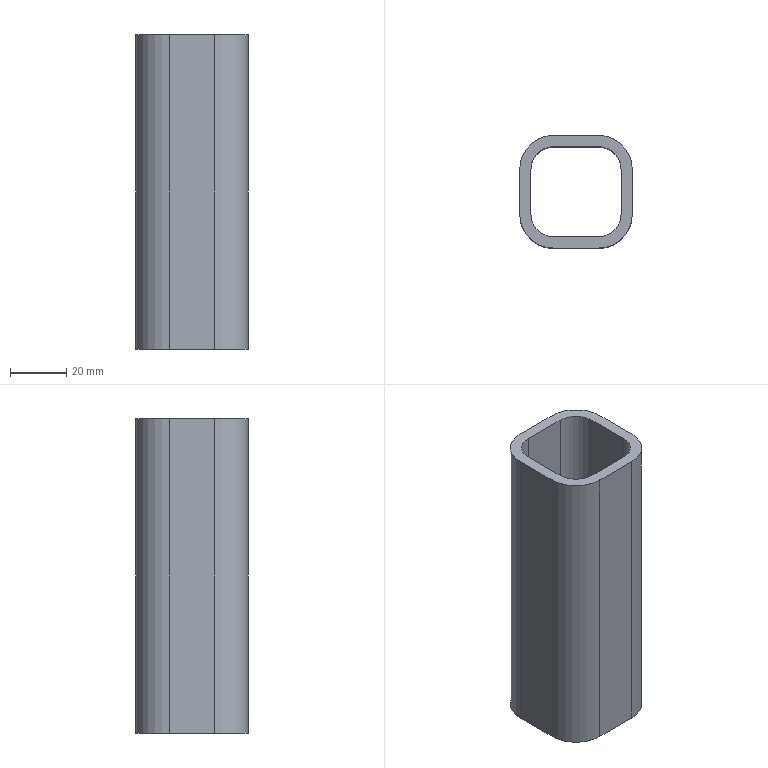Part | SolidWorks | features BaseBody 1 | 1 solid | 18 faces | box 40 x 40 x 111.5 mm | volume 56567 mm3 | plane 10 | cylinder 8 | commonest cylinder face diameters 16 x4 24 x4
STEP:
#1=CARTESIAN_POINT('',(8.,-20.,-31.5));
#2=VERTEX_POINT('',#1);
#3=CARTESIAN_POINT('',(20.,-8.,-31.5));
#4=VERTEX_POINT('',#3);
#5=CARTESIAN_POINT('',(8.,-8.,-31.5));
#6=DIRECTION('',(0.,0.,1.));
#7=DIRECTION('',(1.,0.,0.));
#8=AXIS2_PLACEMENT_3D('',#5,#6,#7);
#9=CIRCLE('',#8,12.);
#10=EDGE_CURVE('',#2,#4,#9,.T.);
#11=ORIENTED_EDGE('',*,*,#10,.T.);
#12=CARTESIAN_POINT('',(20.,-8.,80.));
#13=VERTEX_POINT('',#12);
#14=CARTESIAN_POINT('',(20.,-8.,0.));
#15=DIRECTION('',(0.,0.,1.));
#16=VECTOR('',#15,1000.);
#17=LINE('',#14,#16);
#18=EDGE_CURVE('',#4,#13,#17,.T.);
#19=ORIENTED_EDGE('',*,*,#18,.T.);
#20=CARTESIAN_POINT('',(8.,-20.,80.));
#21=VERTEX_POINT('',#20);
#22=CARTESIAN_POINT('',(8.,-8.,80.));
#23=DIRECTION('',(0.,0.,-1.));
#24=DIRECTION('',(1.,0.,0.));
#25=AXIS2_PLACEMENT_3D('',#22,#23,#24);
#26=CIRCLE('',#25,12.);
#27=EDGE_CURVE('',#13,#21,#26,.T.);
#28=ORIENTED_EDGE('',*,*,#27,.T.);
#29=CARTESIAN_POINT('',(8.,-20.,0.));
#30=DIRECTION('',(0.,0.,-1.));
#31=VECTOR('',#30,1000.);
#32=LINE('',#29,#31);
#33=EDGE_CURVE('',#21,#2,#32,.T.);
#34=ORIENTED_EDGE('',*,*,#33,.T.);
#35=EDGE_LOOP('',(#11,#19,#28,#34));
#36=FACE_OUTER_BOUND('',#35,.T.);
#37=CARTESIAN_POINT('',(8.,-8.,0.));
#38=DIRECTION('',(0.,0.,1.));
#39=DIRECTION('',(1.,0.,0.));
#40=AXIS2_PLACEMENT_3D('',#37,#38,#39);
#41=CYLINDRICAL_SURFACE('',#40,12.);
#42=ADVANCED_FACE('',(#36),#41,.T.);
#43=CARTESIAN_POINT('',(20.,8.,-31.5));
#44=VERTEX_POINT('',#43);
#45=CARTESIAN_POINT('',(20.,8.,-31.5));
#46=DIRECTION('',(0.,1.,0.));
#47=VECTOR('',#46,1000.);
#48=LINE('',#45,#47);
#49=EDGE_CURVE('',#4,#44,#48,.T.);
#50=ORIENTED_EDGE('',*,*,#49,.T.);
#51=CARTESIAN_POINT('',(20.,8.,80.));
#52=VERTEX_POINT('',#51);
#53=CARTESIAN_POINT('',(20.,8.,0.));
#54=DIRECTION('',(0.,0.,1.));
#55=VECTOR('',#54,1000.);
#56=LINE('',#53,#55);
#57=EDGE_CURVE('',#44,#52,#56,.T.);
#58=ORIENTED_EDGE('',*,*,#57,.T.);
#59=CARTESIAN_POINT('',(20.,8.,80.));
#60=DIRECTION('',(0.,-1.,0.));
#61=VECTOR('',#60,1000.);
#62=LINE('',#59,#61);
#63=EDGE_CURVE('',#52,#13,#62,.T.);
#64=ORIENTED_EDGE('',*,*,#63,.T.);
#65=ORIENTED_EDGE('',*,*,#18,.F.);
#66=EDGE_LOOP('',(#50,#58,#64,#65));
#67=FACE_OUTER_BOUND('',#66,.T.);
#68=CARTESIAN_POINT('',(20.,8.,0.));
#69=DIRECTION('',(1.,0.,0.));
#70=DIRECTION('',(0.,1.,0.));
#71=AXIS2_PLACEMENT_3D('',#68,#69,#70);
#72=PLANE('',#71);
#73=ADVANCED_FACE('',(#67),#72,.T.);
#74=CARTESIAN_POINT('',(-16.,8.,-31.5));
#75=VERTEX_POINT('',#74);
#76=CARTESIAN_POINT('',(-8.,16.,-31.5));
#77=VERTEX_POINT('',#76);
#78=CARTESIAN_POINT('',(-8.,8.,-31.5));
#79=DIRECTION('',(0.,0.,-1.));
#80=DIRECTION('',(1.,0.,0.));
#81=AXIS2_PLACEMENT_3D('',#78,#79,#80);
#82=CIRCLE('',#81,8.);
#83=EDGE_CURVE('',#75,#77,#82,.T.);
#84=ORIENTED_EDGE('',*,*,#83,.F.);
#85=CARTESIAN_POINT('',(-16.,-8.,-31.5));
#86=VERTEX_POINT('',#85);
#87=CARTESIAN_POINT('',(-16.,0.,-31.5));
#88=DIRECTION('',(0.,1.,0.));
#89=VECTOR('',#88,1000.);
#90=LINE('',#87,#89);
#91=EDGE_CURVE('',#86,#75,#90,.T.);
#92=ORIENTED_EDGE('',*,*,#91,.F.);
#93=CARTESIAN_POINT('',(-8.,-16.,-31.5));
#94=VERTEX_POINT('',#93);
#95=CARTESIAN_POINT('',(-8.,-8.,-31.5));
#96=DIRECTION('',(0.,0.,-1.));
#97=DIRECTION('',(1.,0.,0.));
#98=AXIS2_PLACEMENT_3D('',#95,#96,#97);
#99=CIRCLE('',#98,8.);
#100=EDGE_CURVE('',#94,#86,#99,.T.);
#101=ORIENTED_EDGE('',*,*,#100,.F.);
#102=CARTESIAN_POINT('',(8.,-16.,-31.5));
#103=VERTEX_POINT('',#102);
#104=CARTESIAN_POINT('',(0.,-16.,-31.5));
#105=DIRECTION('',(-1.,0.,0.));
#106=VECTOR('',#105,1000.);
#107=LINE('',#104,#106);
#108=EDGE_CURVE('',#103,#94,#107,.T.);
#109=ORIENTED_EDGE('',*,*,#108,.F.);
#110=CARTESIAN_POINT('',(16.,-8.,-31.5));
#111=VERTEX_POINT('',#110);
#112=CARTESIAN_POINT('',(8.,-8.,-31.5));
#113=DIRECTION('',(0.,0.,-1.));
#114=DIRECTION('',(1.,0.,0.));
#115=AXIS2_PLACEMENT_3D('',#112,#113,#114);
#116=CIRCLE('',#115,8.);
#117=EDGE_CURVE('',#111,#103,#116,.T.);
#118=ORIENTED_EDGE('',*,*,#117,.F.);
#119=CARTESIAN_POINT('',(16.,8.,-31.5));
#120=VERTEX_POINT('',#119);
#121=CARTESIAN_POINT('',(16.,0.,-31.5));
#122=DIRECTION('',(0.,-1.,0.));
#123=VECTOR('',#122,1000.);
#124=LINE('',#121,#123);
#125=EDGE_CURVE('',#120,#111,#124,.T.);
#126=ORIENTED_EDGE('',*,*,#125,.F.);
#127=CARTESIAN_POINT('',(8.,16.,-31.5));
#128=VERTEX_POINT('',#127);
#129=CARTESIAN_POINT('',(8.,8.,-31.5));
#130=DIRECTION('',(0.,0.,-1.));
#131=DIRECTION('',(1.,0.,0.));
#132=AXIS2_PLACEMENT_3D('',#129,#130,#131);
#133=CIRCLE('',#132,8.);
#134=EDGE_CURVE('',#128,#120,#133,.T.);
#135=ORIENTED_EDGE('',*,*,#134,.F.);
#136=CARTESIAN_POINT('',(0.,16.,-31.5));
#137=DIRECTION('',(1.,0.,0.));
#138=VECTOR('',#137,1000.);
#139=LINE('',#136,#138);
#140=EDGE_CURVE('',#77,#128,#139,.T.);
#141=ORIENTED_EDGE('',*,*,#140,.F.);
#142=EDGE_LOOP('',(#84,#92,#101,#109,#118,#126,#135,#141));
#143=FACE_BOUND('',#142,.T.);
#144=CARTESIAN_POINT('',(-8.,20.,-31.5));
#145=VERTEX_POINT('',#144);
#146=CARTESIAN_POINT('',(-20.,8.,-31.5));
#147=VERTEX_POINT('',#146);
#148=CARTESIAN_POINT('',(-8.,8.,-31.5));
#149=DIRECTION('',(0.,0.,1.));
#150=DIRECTION('',(1.,0.,0.));
#151=AXIS2_PLACEMENT_3D('',#148,#149,#150);
#152=CIRCLE('',#151,12.);
#153=EDGE_CURVE('',#145,#147,#152,.T.);
#154=ORIENTED_EDGE('',*,*,#153,.F.);
#155=CARTESIAN_POINT('',(8.,20.,-31.5));
#156=VERTEX_POINT('',#155);
#157=CARTESIAN_POINT('',(0.,20.,-31.5));
#158=DIRECTION('',(-1.,0.,0.));
#159=VECTOR('',#158,1000.);
#160=LINE('',#157,#159);
#161=EDGE_CURVE('',#156,#145,#160,.T.);
#162=ORIENTED_EDGE('',*,*,#161,.F.);
#163=CARTESIAN_POINT('',(8.,8.,-31.5));
#164=DIRECTION('',(0.,0.,1.));
#165=DIRECTION('',(1.,0.,0.));
#166=AXIS2_PLACEMENT_3D('',#163,#164,#165);
#167=CIRCLE('',#166,12.);
#168=EDGE_CURVE('',#44,#156,#167,.T.);
#169=ORIENTED_EDGE('',*,*,#168,.F.);
#170=ORIENTED_EDGE('',*,*,#49,.F.);
#171=ORIENTED_EDGE('',*,*,#10,.F.);
#172=CARTESIAN_POINT('',(-8.,-20.,-31.5));
#173=VERTEX_POINT('',#172);
#174=CARTESIAN_POINT('',(0.,-20.,-31.5));
#175=DIRECTION('',(1.,0.,0.));
#176=VECTOR('',#175,1000.);
#177=LINE('',#174,#176);
#178=EDGE_CURVE('',#173,#2,#177,.T.);
#179=ORIENTED_EDGE('',*,*,#178,.F.);
#180=CARTESIAN_POINT('',(-20.,-8.,-31.5));
#181=VERTEX_POINT('',#180);
#182=CARTESIAN_POINT('',(-8.,-8.,-31.5));
#183=DIRECTION('',(0.,0.,1.));
#184=DIRECTION('',(1.,0.,0.));
#185=AXIS2_PLACEMENT_3D('',#182,#183,#184);
#186=CIRCLE('',#185,12.);
#187=EDGE_CURVE('',#181,#173,#186,.T.);
#188=ORIENTED_EDGE('',*,*,#187,.F.);
#189=CARTESIAN_POINT('',(-20.,0.,-31.5));
#190=DIRECTION('',(0.,-1.,0.));
#191=VECTOR('',#190,1000.);
#192=LINE('',#189,#191);
#193=EDGE_CURVE('',#147,#181,#192,.T.);
#194=ORIENTED_EDGE('',*,*,#193,.F.);
#195=EDGE_LOOP('',(#154,#162,#169,#170,#171,#179,#188,#194));
#196=FACE_OUTER_BOUND('',#195,.T.);
#197=CARTESIAN_POINT('',(0.,0.,-31.5));
#198=DIRECTION('',(0.,0.,1.));
#199=DIRECTION('',(1.,0.,0.));
#200=AXIS2_PLACEMENT_3D('',#197,#198,#199);
#201=PLANE('',#200);
#202=ADVANCED_FACE('',(#143,#196),#201,.F.);
#203=ORIENTED_EDGE('',*,*,#178,.T.);
#204=ORIENTED_EDGE('',*,*,#33,.F.);
#205=CARTESIAN_POINT('',(-8.,-20.,80.));
#206=VERTEX_POINT('',#205);
#207=CARTESIAN_POINT('',(8.,-20.,80.));
#208=DIRECTION('',(-1.,0.,0.));
#209=VECTOR('',#208,1000.);
#210=LINE('',#207,#209);
#211=EDGE_CURVE('',#21,#206,#210,.T.);
#212=ORIENTED_EDGE('',*,*,#211,.T.);
#213=CARTESIAN_POINT('',(-8.,-20.,0.));
#214=DIRECTION('',(0.,0.,-1.));
#215=VECTOR('',#214,1000.);
#216=LINE('',#213,#215);
#217=EDGE_CURVE('',#206,#173,#216,.T.);
#218=ORIENTED_EDGE('',*,*,#217,.T.);
#219=EDGE_LOOP('',(#203,#204,#212,#218));
#220=FACE_OUTER_BOUND('',#219,.T.);
#221=CARTESIAN_POINT('',(8.,-20.,0.));
#222=DIRECTION('',(0.,-1.,0.));
#223=DIRECTION('',(1.,0.,0.));
#224=AXIS2_PLACEMENT_3D('',#221,#222,#223);
#225=PLANE('',#224);
#226=ADVANCED_FACE('',(#220),#225,.T.);
#227=CARTESIAN_POINT('',(-16.,-8.,80.));
#228=VERTEX_POINT('',#227);
#229=CARTESIAN_POINT('',(-16.,8.,80.));
#230=VERTEX_POINT('',#229);
#231=CARTESIAN_POINT('',(-16.,0.,80.));
#232=DIRECTION('',(0.,1.,0.));
#233=VECTOR('',#232,1000.);
#234=LINE('',#231,#233);
#235=EDGE_CURVE('',#228,#230,#234,.T.);
#236=ORIENTED_EDGE('',*,*,#235,.T.);
#237=CARTESIAN_POINT('',(-8.,16.,80.));
#238=VERTEX_POINT('',#237);
#239=CARTESIAN_POINT('',(-8.,8.,80.));
#240=DIRECTION('',(0.,0.,-1.));
#241=DIRECTION('',(1.,0.,0.));
#242=AXIS2_PLACEMENT_3D('',#239,#240,#241);
#243=CIRCLE('',#242,8.);
#244=EDGE_CURVE('',#230,#238,#243,.T.);
#245=ORIENTED_EDGE('',*,*,#244,.T.);
#246=CARTESIAN_POINT('',(8.,16.,80.));
#247=VERTEX_POINT('',#246);
#248=CARTESIAN_POINT('',(0.,16.,80.));
#249=DIRECTION('',(1.,0.,0.));
#250=VECTOR('',#249,1000.);
#251=LINE('',#248,#250);
#252=EDGE_CURVE('',#238,#247,#251,.T.);
#253=ORIENTED_EDGE('',*,*,#252,.T.);
#254=CARTESIAN_POINT('',(16.,8.,80.));
#255=VERTEX_POINT('',#254);
#256=CARTESIAN_POINT('',(8.,8.,80.));
#257=DIRECTION('',(0.,0.,-1.));
#258=DIRECTION('',(1.,0.,0.));
#259=AXIS2_PLACEMENT_3D('',#256,#257,#258);
#260=CIRCLE('',#259,8.);
#261=EDGE_CURVE('',#247,#255,#260,.T.);
#262=ORIENTED_EDGE('',*,*,#261,.T.);
#263=CARTESIAN_POINT('',(16.,-8.,80.));
#264=VERTEX_POINT('',#263);
#265=CARTESIAN_POINT('',(16.,0.,80.));
#266=DIRECTION('',(0.,-1.,0.));
#267=VECTOR('',#266,1000.);
#268=LINE('',#265,#267);
#269=EDGE_CURVE('',#255,#264,#268,.T.);
#270=ORIENTED_EDGE('',*,*,#269,.T.);
#271=CARTESIAN_POINT('',(8.,-16.,80.));
#272=VERTEX_POINT('',#271);
#273=CARTESIAN_POINT('',(8.,-8.,80.));
#274=DIRECTION('',(0.,0.,-1.));
#275=DIRECTION('',(1.,0.,0.));
#276=AXIS2_PLACEMENT_3D('',#273,#274,#275);
#277=CIRCLE('',#276,8.);
#278=EDGE_CURVE('',#264,#272,#277,.T.);
#279=ORIENTED_EDGE('',*,*,#278,.T.);
#280=CARTESIAN_POINT('',(-8.,-16.,80.));
#281=VERTEX_POINT('',#280);
#282=CARTESIAN_POINT('',(0.,-16.,80.));
#283=DIRECTION('',(-1.,0.,0.));
#284=VECTOR('',#283,1000.);
#285=LINE('',#282,#284);
#286=EDGE_CURVE('',#272,#281,#285,.T.);
#287=ORIENTED_EDGE('',*,*,#286,.T.);
#288=CARTESIAN_POINT('',(-8.,-8.,80.));
#289=DIRECTION('',(0.,0.,-1.));
#290=DIRECTION('',(1.,0.,0.));
#291=AXIS2_PLACEMENT_3D('',#288,#289,#290);
#292=CIRCLE('',#291,8.);
#293=EDGE_CURVE('',#281,#228,#292,.T.);
#294=ORIENTED_EDGE('',*,*,#293,.T.);
#295=EDGE_LOOP('',(#236,#245,#253,#262,#270,#279,#287,#294));
#296=FACE_BOUND('',#295,.T.);
#297=CARTESIAN_POINT('',(8.,20.,80.));
#298=VERTEX_POINT('',#297);
#299=CARTESIAN_POINT('',(-8.,20.,80.));
#300=VERTEX_POINT('',#299);
#301=CARTESIAN_POINT('',(0.,20.,80.));
#302=DIRECTION('',(-1.,0.,0.));
#303=VECTOR('',#302,1000.);
#304=LINE('',#301,#303);
#305=EDGE_CURVE('',#298,#300,#304,.T.);
#306=ORIENTED_EDGE('',*,*,#305,.T.);
#307=CARTESIAN_POINT('',(-20.,8.,80.));
#308=VERTEX_POINT('',#307);
#309=CARTESIAN_POINT('',(-8.,8.,80.));
#310=DIRECTION('',(0.,0.,1.));
#311=DIRECTION('',(1.,0.,0.));
#312=AXIS2_PLACEMENT_3D('',#309,#310,#311);
#313=CIRCLE('',#312,12.);
#314=EDGE_CURVE('',#300,#308,#313,.T.);
#315=ORIENTED_EDGE('',*,*,#314,.T.);
#316=CARTESIAN_POINT('',(-20.,-8.,80.));
#317=VERTEX_POINT('',#316);
#318=CARTESIAN_POINT('',(-20.,0.,80.));
#319=DIRECTION('',(0.,-1.,0.));
#320=VECTOR('',#319,1000.);
#321=LINE('',#318,#320);
#322=EDGE_CURVE('',#308,#317,#321,.T.);
#323=ORIENTED_EDGE('',*,*,#322,.T.);
#324=CARTESIAN_POINT('',(-8.,-8.,80.));
#325=DIRECTION('',(0.,0.,1.));
#326=DIRECTION('',(1.,0.,0.));
#327=AXIS2_PLACEMENT_3D('',#324,#325,#326);
#328=CIRCLE('',#327,12.);
#329=EDGE_CURVE('',#317,#206,#328,.T.);
#330=ORIENTED_EDGE('',*,*,#329,.T.);
#331=ORIENTED_EDGE('',*,*,#211,.F.);
#332=ORIENTED_EDGE('',*,*,#27,.F.);
#333=ORIENTED_EDGE('',*,*,#63,.F.);
#334=CARTESIAN_POINT('',(8.,8.,80.));
#335=DIRECTION('',(0.,0.,1.));
#336=DIRECTION('',(1.,0.,0.));
#337=AXIS2_PLACEMENT_3D('',#334,#335,#336);
#338=CIRCLE('',#337,12.);
#339=EDGE_CURVE('',#52,#298,#338,.T.);
#340=ORIENTED_EDGE('',*,*,#339,.T.);
#341=EDGE_LOOP('',(#306,#315,#323,#330,#331,#332,#333,#340));
#342=FACE_OUTER_BOUND('',#341,.T.);
#343=CARTESIAN_POINT('',(0.,0.,80.));
#344=DIRECTION('',(0.,0.,1.));
#345=DIRECTION('',(1.,0.,0.));
#346=AXIS2_PLACEMENT_3D('',#343,#344,#345);
#347=PLANE('',#346);
#348=ADVANCED_FACE('',(#296,#342),#347,.T.);
#349=ORIENTED_EDGE('',*,*,#168,.T.);
#350=CARTESIAN_POINT('',(8.,20.,0.));
#351=DIRECTION('',(0.,0.,1.));
#352=VECTOR('',#351,1000.);
#353=LINE('',#350,#352);
#354=EDGE_CURVE('',#156,#298,#353,.T.);
#355=ORIENTED_EDGE('',*,*,#354,.T.);
#356=ORIENTED_EDGE('',*,*,#339,.F.);
#357=ORIENTED_EDGE('',*,*,#57,.F.);
#358=EDGE_LOOP('',(#349,#355,#356,#357));
#359=FACE_OUTER_BOUND('',#358,.T.);
#360=CARTESIAN_POINT('',(8.,8.,0.));
#361=DIRECTION('',(0.,0.,1.));
#362=DIRECTION('',(1.,0.,0.));
#363=AXIS2_PLACEMENT_3D('',#360,#361,#362);
#364=CYLINDRICAL_SURFACE('',#363,12.);
#365=ADVANCED_FACE('',(#359),#364,.T.);
#366=CARTESIAN_POINT('',(-8.,16.,0.));
#367=DIRECTION('',(0.,0.,1.));
#368=VECTOR('',#367,1000.);
#369=LINE('',#366,#368);
#370=EDGE_CURVE('',#77,#238,#369,.T.);
#371=ORIENTED_EDGE('',*,*,#370,.F.);
#372=ORIENTED_EDGE('',*,*,#140,.T.);
#373=CARTESIAN_POINT('',(8.,16.,0.));
#374=DIRECTION('',(0.,0.,-1.));
#375=VECTOR('',#374,1000.);
#376=LINE('',#373,#375);
#377=EDGE_CURVE('',#247,#128,#376,.T.);
#378=ORIENTED_EDGE('',*,*,#377,.F.);
#379=ORIENTED_EDGE('',*,*,#252,.F.);
#380=EDGE_LOOP('',(#371,#372,#378,#379));
#381=FACE_OUTER_BOUND('',#380,.T.);
#382=CARTESIAN_POINT('',(-8.,16.,0.));
#383=DIRECTION('',(0.,1.,0.));
#384=DIRECTION('',(-1.,0.,0.));
#385=AXIS2_PLACEMENT_3D('',#382,#383,#384);
#386=PLANE('',#385);
#387=ADVANCED_FACE('',(#381),#386,.F.);
#388=CARTESIAN_POINT('',(-16.,8.,0.));
#389=DIRECTION('',(0.,0.,1.));
#390=VECTOR('',#389,1000.);
#391=LINE('',#388,#390);
#392=EDGE_CURVE('',#75,#230,#391,.T.);
#393=ORIENTED_EDGE('',*,*,#392,.F.);
#394=ORIENTED_EDGE('',*,*,#83,.T.);
#395=ORIENTED_EDGE('',*,*,#370,.T.);
#396=ORIENTED_EDGE('',*,*,#244,.F.);
#397=EDGE_LOOP('',(#393,#394,#395,#396));
#398=FACE_OUTER_BOUND('',#397,.T.);
#399=CARTESIAN_POINT('',(-8.,8.,0.));
#400=DIRECTION('',(0.,0.,1.));
#401=DIRECTION('',(1.,0.,0.));
#402=AXIS2_PLACEMENT_3D('',#399,#400,#401);
#403=CYLINDRICAL_SURFACE('',#402,8.);
#404=ADVANCED_FACE('',(#398),#403,.F.);
#405=CARTESIAN_POINT('',(-16.,-8.,0.));
#406=DIRECTION('',(0.,0.,1.));
#407=VECTOR('',#406,1000.);
#408=LINE('',#405,#407);
#409=EDGE_CURVE('',#86,#228,#408,.T.);
#410=ORIENTED_EDGE('',*,*,#409,.F.);
#411=ORIENTED_EDGE('',*,*,#91,.T.);
#412=ORIENTED_EDGE('',*,*,#392,.T.);
#413=ORIENTED_EDGE('',*,*,#235,.F.);
#414=EDGE_LOOP('',(#410,#411,#412,#413));
#415=FACE_OUTER_BOUND('',#414,.T.);
#416=CARTESIAN_POINT('',(-16.,-8.,0.));
#417=DIRECTION('',(-1.,0.,0.));
#418=DIRECTION('',(0.,-1.,0.));
#419=AXIS2_PLACEMENT_3D('',#416,#417,#418);
#420=PLANE('',#419);
#421=ADVANCED_FACE('',(#415),#420,.F.);
#422=CARTESIAN_POINT('',(-8.,-16.,0.));
#423=DIRECTION('',(0.,0.,1.));
#424=VECTOR('',#423,1000.);
#425=LINE('',#422,#424);
#426=EDGE_CURVE('',#94,#281,#425,.T.);
#427=ORIENTED_EDGE('',*,*,#426,.F.);
#428=ORIENTED_EDGE('',*,*,#100,.T.);
#429=ORIENTED_EDGE('',*,*,#409,.T.);
#430=ORIENTED_EDGE('',*,*,#293,.F.);
#431=EDGE_LOOP('',(#427,#428,#429,#430));
#432=FACE_OUTER_BOUND('',#431,.T.);
#433=CARTESIAN_POINT('',(-8.,-8.,0.));
#434=DIRECTION('',(0.,0.,1.));
#435=DIRECTION('',(1.,0.,0.));
#436=AXIS2_PLACEMENT_3D('',#433,#434,#435);
#437=CYLINDRICAL_SURFACE('',#436,8.);
#438=ADVANCED_FACE('',(#432),#437,.F.);
#439=CARTESIAN_POINT('',(8.,-16.,0.));
#440=DIRECTION('',(0.,0.,1.));
#441=VECTOR('',#440,1000.);
#442=LINE('',#439,#441);
#443=EDGE_CURVE('',#103,#272,#442,.T.);
#444=ORIENTED_EDGE('',*,*,#443,.F.);
#445=ORIENTED_EDGE('',*,*,#108,.T.);
#446=ORIENTED_EDGE('',*,*,#426,.T.);
#447=ORIENTED_EDGE('',*,*,#286,.F.);
#448=EDGE_LOOP('',(#444,#445,#446,#447));
#449=FACE_OUTER_BOUND('',#448,.T.);
#450=CARTESIAN_POINT('',(8.,-16.,0.));
#451=DIRECTION('',(0.,-1.,0.));
#452=DIRECTION('',(1.,0.,0.));
#453=AXIS2_PLACEMENT_3D('',#450,#451,#452);
#454=PLANE('',#453);
#455=ADVANCED_FACE('',(#449),#454,.F.);
#456=CARTESIAN_POINT('',(16.,-8.,0.));
#457=DIRECTION('',(0.,0.,1.));
#458=VECTOR('',#457,1000.);
#459=LINE('',#456,#458);
#460=EDGE_CURVE('',#111,#264,#459,.T.);
#461=ORIENTED_EDGE('',*,*,#460,.F.);
#462=ORIENTED_EDGE('',*,*,#117,.T.);
#463=ORIENTED_EDGE('',*,*,#443,.T.);
#464=ORIENTED_EDGE('',*,*,#278,.F.);
#465=EDGE_LOOP('',(#461,#462,#463,#464));
#466=FACE_OUTER_BOUND('',#465,.T.);
#467=CARTESIAN_POINT('',(8.,-8.,0.));
#468=DIRECTION('',(0.,0.,1.));
#469=DIRECTION('',(1.,0.,0.));
#470=AXIS2_PLACEMENT_3D('',#467,#468,#469);
#471=CYLINDRICAL_SURFACE('',#470,8.);
#472=ADVANCED_FACE('',(#466),#471,.F.);
#473=CARTESIAN_POINT('',(16.,8.,0.));
#474=DIRECTION('',(0.,0.,1.));
#475=VECTOR('',#474,1000.);
#476=LINE('',#473,#475);
#477=EDGE_CURVE('',#120,#255,#476,.T.);
#478=ORIENTED_EDGE('',*,*,#477,.F.);
#479=ORIENTED_EDGE('',*,*,#125,.T.);
#480=ORIENTED_EDGE('',*,*,#460,.T.);
#481=ORIENTED_EDGE('',*,*,#269,.F.);
#482=EDGE_LOOP('',(#478,#479,#480,#481));
#483=FACE_OUTER_BOUND('',#482,.T.);
#484=CARTESIAN_POINT('',(16.,8.,0.));
#485=DIRECTION('',(1.,0.,0.));
#486=DIRECTION('',(0.,0.,-1.));
#487=AXIS2_PLACEMENT_3D('',#484,#485,#486);
#488=PLANE('',#487);
#489=ADVANCED_FACE('',(#483),#488,.F.);
#490=ORIENTED_EDGE('',*,*,#377,.T.);
#491=ORIENTED_EDGE('',*,*,#134,.T.);
#492=ORIENTED_EDGE('',*,*,#477,.T.);
#493=ORIENTED_EDGE('',*,*,#261,.F.);
#494=EDGE_LOOP('',(#490,#491,#492,#493));
#495=FACE_OUTER_BOUND('',#494,.T.);
#496=CARTESIAN_POINT('',(8.,8.,0.));
#497=DIRECTION('',(0.,0.,1.));
#498=DIRECTION('',(1.,0.,0.));
#499=AXIS2_PLACEMENT_3D('',#496,#497,#498);
#500=CYLINDRICAL_SURFACE('',#499,8.);
#501=ADVANCED_FACE('',(#495),#500,.F.);
#502=ORIENTED_EDGE('',*,*,#193,.T.);
#503=CARTESIAN_POINT('',(-20.,-8.,0.));
#504=DIRECTION('',(0.,0.,1.));
#505=VECTOR('',#504,1000.);
#506=LINE('',#503,#505);
#507=EDGE_CURVE('',#181,#317,#506,.T.);
#508=ORIENTED_EDGE('',*,*,#507,.T.);
#509=ORIENTED_EDGE('',*,*,#322,.F.);
#510=CARTESIAN_POINT('',(-20.,8.,0.));
#511=DIRECTION('',(0.,0.,-1.));
#512=VECTOR('',#511,1000.);
#513=LINE('',#510,#512);
#514=EDGE_CURVE('',#308,#147,#513,.T.);
#515=ORIENTED_EDGE('',*,*,#514,.T.);
#516=EDGE_LOOP('',(#502,#508,#509,#515));
#517=FACE_OUTER_BOUND('',#516,.T.);
#518=CARTESIAN_POINT('',(-20.,-8.,0.));
#519=DIRECTION('',(-1.,0.,0.));
#520=DIRECTION('',(0.,-1.,0.));
#521=AXIS2_PLACEMENT_3D('',#518,#519,#520);
#522=PLANE('',#521);
#523=ADVANCED_FACE('',(#517),#522,.T.);
#524=ORIENTED_EDGE('',*,*,#153,.T.);
#525=ORIENTED_EDGE('',*,*,#514,.F.);
#526=ORIENTED_EDGE('',*,*,#314,.F.);
#527=CARTESIAN_POINT('',(-8.,20.,0.));
#528=DIRECTION('',(0.,0.,-1.));
#529=VECTOR('',#528,1000.);
#530=LINE('',#527,#529);
#531=EDGE_CURVE('',#300,#145,#530,.T.);
#532=ORIENTED_EDGE('',*,*,#531,.T.);
#533=EDGE_LOOP('',(#524,#525,#526,#532));
#534=FACE_OUTER_BOUND('',#533,.T.);
#535=CARTESIAN_POINT('',(-8.,8.,0.));
#536=DIRECTION('',(0.,0.,1.));
#537=DIRECTION('',(1.,0.,0.));
#538=AXIS2_PLACEMENT_3D('',#535,#536,#537);
#539=CYLINDRICAL_SURFACE('',#538,12.);
#540=ADVANCED_FACE('',(#534),#539,.T.);
#541=ORIENTED_EDGE('',*,*,#161,.T.);
#542=ORIENTED_EDGE('',*,*,#531,.F.);
#543=ORIENTED_EDGE('',*,*,#305,.F.);
#544=ORIENTED_EDGE('',*,*,#354,.F.);
#545=EDGE_LOOP('',(#541,#542,#543,#544));
#546=FACE_OUTER_BOUND('',#545,.T.);
#547=CARTESIAN_POINT('',(-8.,20.,0.));
#548=DIRECTION('',(0.,1.,0.));
#549=DIRECTION('',(0.,0.,1.));
#550=AXIS2_PLACEMENT_3D('',#547,#548,#549);
#551=PLANE('',#550);
#552=ADVANCED_FACE('',(#546),#551,.T.);
#553=ORIENTED_EDGE('',*,*,#187,.T.);
#554=ORIENTED_EDGE('',*,*,#217,.F.);
#555=ORIENTED_EDGE('',*,*,#329,.F.);
#556=ORIENTED_EDGE('',*,*,#507,.F.);
#557=EDGE_LOOP('',(#553,#554,#555,#556));
#558=FACE_OUTER_BOUND('',#557,.T.);
#559=CARTESIAN_POINT('',(-8.,-8.,0.));
#560=DIRECTION('',(0.,0.,1.));
#561=DIRECTION('',(1.,0.,0.));
#562=AXIS2_PLACEMENT_3D('',#559,#560,#561);
#563=CYLINDRICAL_SURFACE('',#562,12.);
#564=ADVANCED_FACE('',(#558),#563,.T.);
#565=CLOSED_SHELL('',(#42,#73,#202,#226,#348,#365,#387,#404,#421,#438,#455,#472,#489,#501,#523,#540,#552,#564));
#566=MANIFOLD_SOLID_BREP('',#565);
#567=CARTESIAN_POINT('',(0.,0.,0.));
#568=DIRECTION('',(0.,0.,1.));
#569=DIRECTION('',(1.,0.,0.));
#570=AXIS2_PLACEMENT_3D('',#567,#568,#569);
#571=(LENGTH_UNIT()NAMED_UNIT(*)SI_UNIT(.MILLI.,.METRE.));
#572=UNCERTAINTY_MEASURE_WITH_UNIT(LENGTH_MEASURE(0.00001),#571,'','');
#573=(NAMED_UNIT(*)PLANE_ANGLE_UNIT()SI_UNIT($,.RADIAN.));
#574=(NAMED_UNIT(*)SI_UNIT($,.STERADIAN.)SOLID_ANGLE_UNIT());
#575=(GEOMETRIC_REPRESENTATION_CONTEXT(3)GLOBAL_UNCERTAINTY_ASSIGNED_CONTEXT((#572))GLOBAL_UNIT_ASSIGNED_CONTEXT((#571,#573,#574))REPRESENTATION_CONTEXT('',''));
#576=ADVANCED_BREP_SHAPE_REPRESENTATION('',(#566,#570),#575);